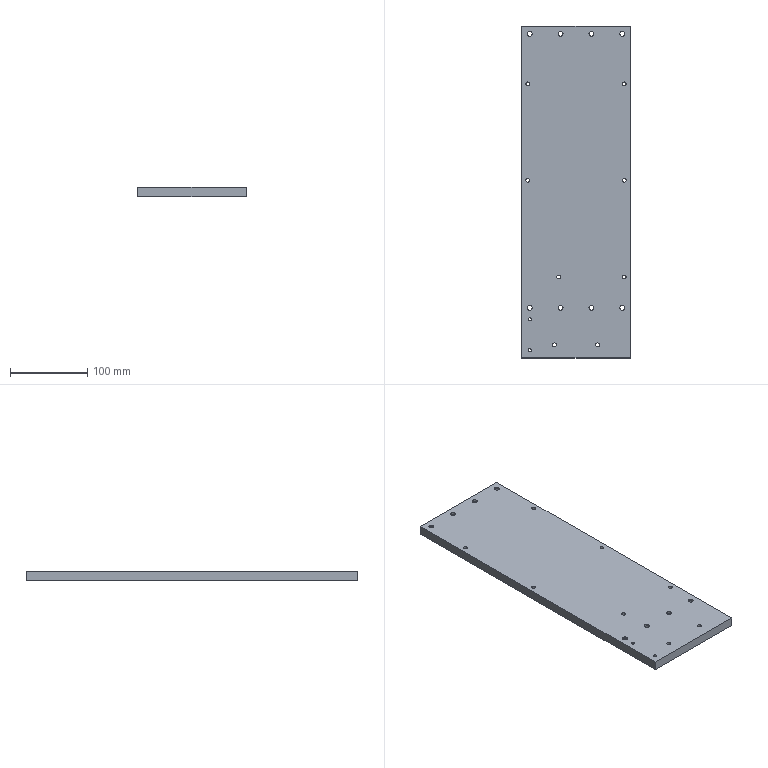Part | STEP file | 0232_201_Base_Plate | 1 solid | 66 faces | box 140 x 430 x 12 mm | volume 707820 mm3 | cylinder 52 | plane 14 | commonest cylinder face diameters 5 x16 6.5 x16 14 x16 4.2 x4